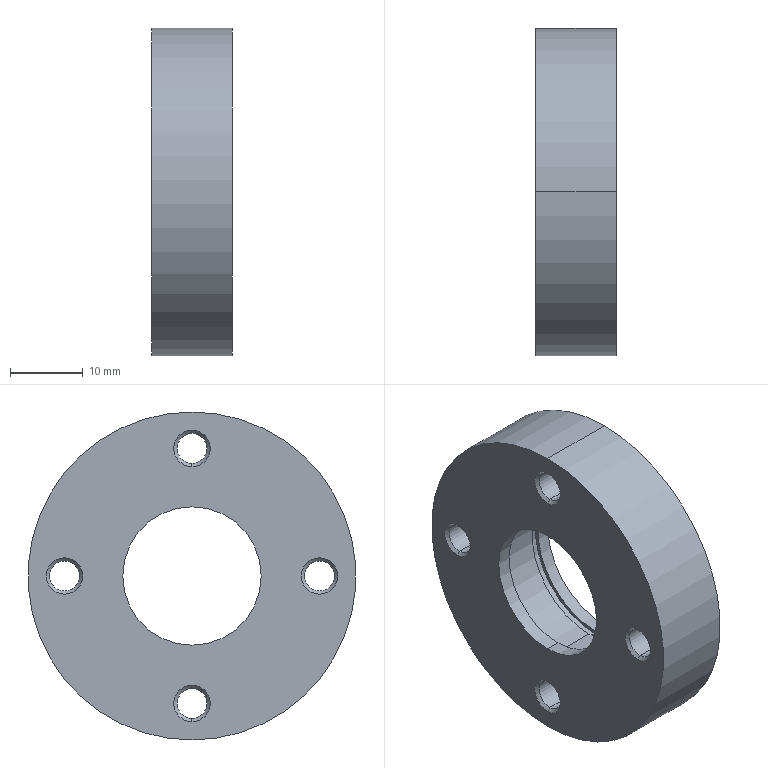Part | STEP file | Bearing seat BGRAB6900DD_h V1.201001 | 1 solid | 51 faces | box 11 x 45 x 45 mm | volume 12216 mm3 | cylinder 26 | cone 16 | plane 9 | commonest cylinder face diameters 4.134 x8 8 x8 22 x4 19 x2 23 x2 45 x2